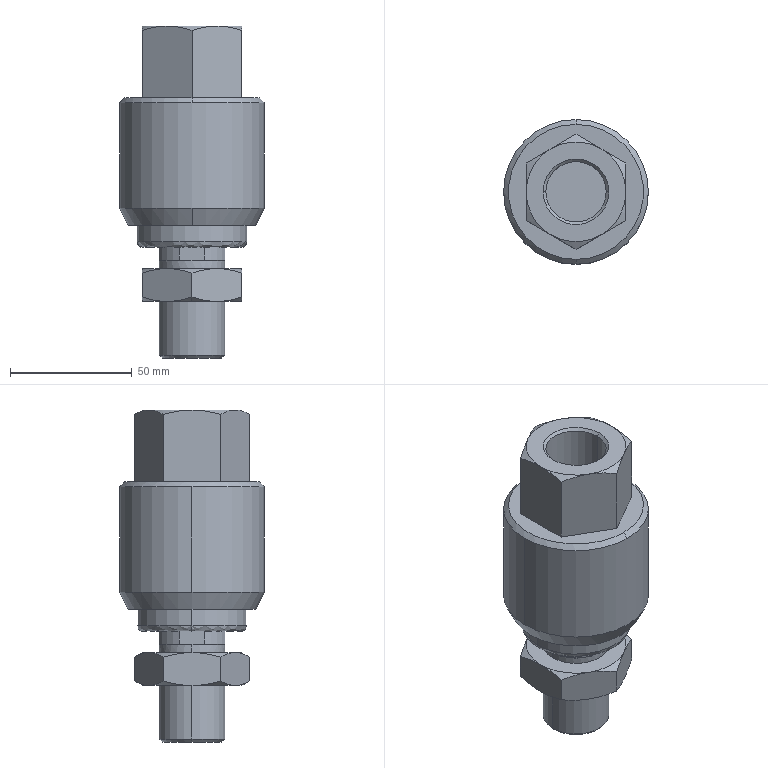Part | SolidWorks | features BaseBody 1 | 1 solid | 84 faces | box 59.5 x 59.5 x 136.5 mm | volume 218418 mm3 | cone 37 | plane 31 | cylinder 14 | spline 2 | commonest cylinder face diameters 27 x4 29 x4 24.835 x2 45 x2 59.5 x2